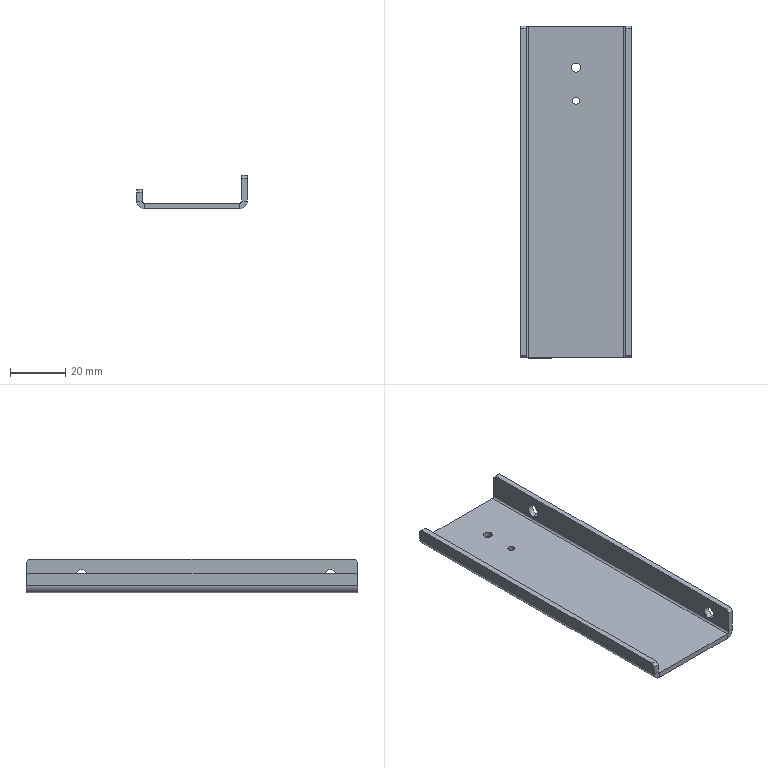Part | NX | features BREP 1 | 1 solid | 34 faces | box 40 x 120 x 12 mm | volume 12748 mm3 | plane 22 | cylinder 12 | commonest cylinder face diameters 4.5 x4 1.473 x2 2.5 x2 3.3 x2 5.473 x2
STEP:
#1=CARTESIAN_POINT('',(16.75,93.,-2.));
#2=VERTEX_POINT('',#1);
#3=CARTESIAN_POINT('',(19.25,93.,-2.));
#4=VERTEX_POINT('',#3);
#5=CARTESIAN_POINT('',(18.,93.,-2.));
#6=DIRECTION('',(0.,0.,1.));
#7=DIRECTION('',(1.,0.,0.));
#8=AXIS2_PLACEMENT_3D('',#5,#6,#7);
#9=CIRCLE('',#8,1.25);
#10=EDGE_CURVE('',#2,#4,#9,.T.);
#11=ORIENTED_EDGE('',*,*,#10,.F.);
#12=CARTESIAN_POINT('',(16.75,93.,0.));
#13=VERTEX_POINT('',#12);
#14=CARTESIAN_POINT('',(16.75,93.,0.));
#15=DIRECTION('',(0.,0.,1.));
#16=VECTOR('',#15,1000.);
#17=LINE('',#14,#16);
#18=EDGE_CURVE('',#13,#2,#17,.F.);
#19=ORIENTED_EDGE('',*,*,#18,.F.);
#20=CARTESIAN_POINT('',(19.25,93.,0.));
#21=VERTEX_POINT('',#20);
#22=CARTESIAN_POINT('',(18.,93.,0.));
#23=DIRECTION('',(0.,0.,1.));
#24=DIRECTION('',(1.,0.,0.));
#25=AXIS2_PLACEMENT_3D('',#22,#23,#24);
#26=CIRCLE('',#25,1.25);
#27=EDGE_CURVE('',#13,#21,#26,.T.);
#28=ORIENTED_EDGE('',*,*,#27,.T.);
#29=CARTESIAN_POINT('',(19.25,93.,0.));
#30=DIRECTION('',(0.,0.,1.));
#31=VECTOR('',#30,1000.);
#32=LINE('',#29,#31);
#33=EDGE_CURVE('',#21,#4,#32,.F.);
#34=ORIENTED_EDGE('',*,*,#33,.T.);
#35=EDGE_LOOP('',(#11,#19,#28,#34));
#36=FACE_BOUND('',#35,.T.);
#37=CARTESIAN_POINT('',(18.,93.,0.));
#38=DIRECTION('',(0.,0.,1.));
#39=DIRECTION('',(1.,0.,0.));
#40=AXIS2_PLACEMENT_3D('',#37,#38,#39);
#41=CYLINDRICAL_SURFACE('',#40,1.25);
#42=ADVANCED_FACE('',(#36),#41,.F.);
#43=CARTESIAN_POINT('',(16.35,105.,-2.));
#44=VERTEX_POINT('',#43);
#45=CARTESIAN_POINT('',(19.65,105.,-2.));
#46=VERTEX_POINT('',#45);
#47=CARTESIAN_POINT('',(18.,105.,-2.));
#48=DIRECTION('',(0.,0.,1.));
#49=DIRECTION('',(1.,0.,0.));
#50=AXIS2_PLACEMENT_3D('',#47,#48,#49);
#51=CIRCLE('',#50,1.65);
#52=EDGE_CURVE('',#44,#46,#51,.T.);
#53=ORIENTED_EDGE('',*,*,#52,.F.);
#54=CARTESIAN_POINT('',(16.35,105.,0.));
#55=VERTEX_POINT('',#54);
#56=CARTESIAN_POINT('',(16.35,105.,0.));
#57=DIRECTION('',(0.,0.,1.));
#58=VECTOR('',#57,1000.);
#59=LINE('',#56,#58);
#60=EDGE_CURVE('',#55,#44,#59,.F.);
#61=ORIENTED_EDGE('',*,*,#60,.F.);
#62=CARTESIAN_POINT('',(19.65,105.,0.));
#63=VERTEX_POINT('',#62);
#64=CARTESIAN_POINT('',(18.,105.,0.));
#65=DIRECTION('',(0.,0.,1.));
#66=DIRECTION('',(1.,0.,0.));
#67=AXIS2_PLACEMENT_3D('',#64,#65,#66);
#68=CIRCLE('',#67,1.65);
#69=EDGE_CURVE('',#55,#63,#68,.T.);
#70=ORIENTED_EDGE('',*,*,#69,.T.);
#71=CARTESIAN_POINT('',(19.65,105.,0.));
#72=DIRECTION('',(0.,0.,1.));
#73=VECTOR('',#72,1000.);
#74=LINE('',#71,#73);
#75=EDGE_CURVE('',#63,#46,#74,.F.);
#76=ORIENTED_EDGE('',*,*,#75,.T.);
#77=EDGE_LOOP('',(#53,#61,#70,#76));
#78=FACE_BOUND('',#77,.T.);
#79=CARTESIAN_POINT('',(18.,105.,0.));
#80=DIRECTION('',(0.,0.,1.));
#81=DIRECTION('',(1.,0.,0.));
#82=AXIS2_PLACEMENT_3D('',#79,#80,#81);
#83=CYLINDRICAL_SURFACE('',#82,1.65);
#84=ADVANCED_FACE('',(#78),#83,.F.);
#85=CARTESIAN_POINT('',(36.,100.,1.75));
#86=VERTEX_POINT('',#85);
#87=CARTESIAN_POINT('',(36.,100.,6.25));
#88=VERTEX_POINT('',#87);
#89=CARTESIAN_POINT('',(36.,100.,4.));
#90=DIRECTION('',(-1.,0.,0.));
#91=DIRECTION('',(0.,0.,1.));
#92=AXIS2_PLACEMENT_3D('',#89,#90,#91);
#93=CIRCLE('',#92,2.25);
#94=EDGE_CURVE('',#86,#88,#93,.T.);
#95=ORIENTED_EDGE('',*,*,#94,.T.);
#96=CARTESIAN_POINT('',(38.,100.,6.25));
#97=VERTEX_POINT('',#96);
#98=CARTESIAN_POINT('',(38.,100.,6.25));
#99=DIRECTION('',(1.,0.,0.));
#100=VECTOR('',#99,1000.);
#101=LINE('',#98,#100);
#102=EDGE_CURVE('',#88,#97,#101,.T.);
#103=ORIENTED_EDGE('',*,*,#102,.T.);
#104=CARTESIAN_POINT('',(38.,100.,1.75));
#105=VERTEX_POINT('',#104);
#106=CARTESIAN_POINT('',(38.,100.,4.));
#107=DIRECTION('',(1.,0.,0.));
#108=DIRECTION('',(0.,0.,-1.));
#109=AXIS2_PLACEMENT_3D('',#106,#107,#108);
#110=CIRCLE('',#109,2.25);
#111=EDGE_CURVE('',#97,#105,#110,.T.);
#112=ORIENTED_EDGE('',*,*,#111,.T.);
#113=CARTESIAN_POINT('',(38.,100.,1.75));
#114=DIRECTION('',(1.,0.,0.));
#115=VECTOR('',#114,1000.);
#116=LINE('',#113,#115);
#117=EDGE_CURVE('',#86,#105,#116,.T.);
#118=ORIENTED_EDGE('',*,*,#117,.F.);
#119=EDGE_LOOP('',(#95,#103,#112,#118));
#120=FACE_BOUND('',#119,.T.);
#121=CARTESIAN_POINT('',(38.,100.,4.));
#122=DIRECTION('',(1.,0.,0.));
#123=DIRECTION('',(0.,0.,-1.));
#124=AXIS2_PLACEMENT_3D('',#121,#122,#123);
#125=CYLINDRICAL_SURFACE('',#124,2.25);
#126=ADVANCED_FACE('',(#120),#125,.F.);
#127=CARTESIAN_POINT('',(36.,10.,1.75));
#128=VERTEX_POINT('',#127);
#129=CARTESIAN_POINT('',(36.,10.,6.25));
#130=VERTEX_POINT('',#129);
#131=CARTESIAN_POINT('',(36.,10.,4.));
#132=DIRECTION('',(-1.,0.,0.));
#133=DIRECTION('',(0.,0.,1.));
#134=AXIS2_PLACEMENT_3D('',#131,#132,#133);
#135=CIRCLE('',#134,2.25);
#136=EDGE_CURVE('',#128,#130,#135,.T.);
#137=ORIENTED_EDGE('',*,*,#136,.T.);
#138=CARTESIAN_POINT('',(38.,10.,6.25));
#139=VERTEX_POINT('',#138);
#140=CARTESIAN_POINT('',(38.,10.,6.25));
#141=DIRECTION('',(1.,0.,0.));
#142=VECTOR('',#141,1000.);
#143=LINE('',#140,#142);
#144=EDGE_CURVE('',#130,#139,#143,.T.);
#145=ORIENTED_EDGE('',*,*,#144,.T.);
#146=CARTESIAN_POINT('',(38.,10.,1.75));
#147=VERTEX_POINT('',#146);
#148=CARTESIAN_POINT('',(38.,10.,4.));
#149=DIRECTION('',(1.,0.,0.));
#150=DIRECTION('',(0.,0.,-1.));
#151=AXIS2_PLACEMENT_3D('',#148,#149,#150);
#152=CIRCLE('',#151,2.25);
#153=EDGE_CURVE('',#139,#147,#152,.T.);
#154=ORIENTED_EDGE('',*,*,#153,.T.);
#155=CARTESIAN_POINT('',(38.,10.,1.75));
#156=DIRECTION('',(1.,0.,0.));
#157=VECTOR('',#156,1000.);
#158=LINE('',#155,#157);
#159=EDGE_CURVE('',#128,#147,#158,.T.);
#160=ORIENTED_EDGE('',*,*,#159,.F.);
#161=EDGE_LOOP('',(#137,#145,#154,#160));
#162=FACE_BOUND('',#161,.T.);
#163=CARTESIAN_POINT('',(38.,10.,4.));
#164=DIRECTION('',(1.,0.,0.));
#165=DIRECTION('',(0.,0.,-1.));
#166=AXIS2_PLACEMENT_3D('',#163,#164,#165);
#167=CYLINDRICAL_SURFACE('',#166,2.25);
#168=ADVANCED_FACE('',(#162),#167,.F.);
#169=CARTESIAN_POINT('',(38.,119.,10.));
#170=VERTEX_POINT('',#169);
#171=CARTESIAN_POINT('',(38.,1.,10.));
#172=VERTEX_POINT('',#171);
#173=CARTESIAN_POINT('',(38.,0.,10.));
#174=DIRECTION('',(0.,-1.,0.));
#175=VECTOR('',#174,1000.);
#176=LINE('',#173,#175);
#177=EDGE_CURVE('',#170,#172,#176,.T.);
#178=ORIENTED_EDGE('',*,*,#177,.T.);
#179=CARTESIAN_POINT('',(38.,0.,9.));
#180=VERTEX_POINT('',#179);
#181=CARTESIAN_POINT('',(38.,0.,9.));
#182=DIRECTION('',(0.,-0.7071,-0.7071));
#183=VECTOR('',#182,1000.);
#184=LINE('',#181,#183);
#185=EDGE_CURVE('',#172,#180,#184,.T.);
#186=ORIENTED_EDGE('',*,*,#185,.T.);
#187=CARTESIAN_POINT('',(38.,0.,0.7366));
#188=VERTEX_POINT('',#187);
#189=CARTESIAN_POINT('',(38.,0.,0.));
#190=DIRECTION('',(0.,0.,-1.));
#191=VECTOR('',#190,1000.);
#192=LINE('',#189,#191);
#193=EDGE_CURVE('',#180,#188,#192,.T.);
#194=ORIENTED_EDGE('',*,*,#193,.T.);
#195=CARTESIAN_POINT('',(38.,120.,0.7366));
#196=VERTEX_POINT('',#195);
#197=CARTESIAN_POINT('',(38.,0.,0.7366));
#198=DIRECTION('',(0.,-1.,0.));
#199=VECTOR('',#198,1000.);
#200=LINE('',#197,#199);
#201=EDGE_CURVE('',#196,#188,#200,.T.);
#202=ORIENTED_EDGE('',*,*,#201,.F.);
#203=CARTESIAN_POINT('',(38.,120.,9.));
#204=VERTEX_POINT('',#203);
#205=CARTESIAN_POINT('',(38.,120.,10.));
#206=DIRECTION('',(0.,0.,1.));
#207=VECTOR('',#206,1000.);
#208=LINE('',#205,#207);
#209=EDGE_CURVE('',#196,#204,#208,.T.);
#210=ORIENTED_EDGE('',*,*,#209,.T.);
#211=CARTESIAN_POINT('',(38.,119.,10.));
#212=DIRECTION('',(0.,-0.7071,0.7071));
#213=VECTOR('',#212,1000.);
#214=LINE('',#211,#213);
#215=EDGE_CURVE('',#204,#170,#214,.T.);
#216=ORIENTED_EDGE('',*,*,#215,.T.);
#217=EDGE_LOOP('',(#178,#186,#194,#202,#210,#216));
#218=FACE_BOUND('',#217,.T.);
#219=CARTESIAN_POINT('',(38.,10.,4.));
#220=DIRECTION('',(1.,0.,0.));
#221=DIRECTION('',(0.,0.,-1.));
#222=AXIS2_PLACEMENT_3D('',#219,#220,#221);
#223=CIRCLE('',#222,2.25);
#224=EDGE_CURVE('',#147,#139,#223,.T.);
#225=ORIENTED_EDGE('',*,*,#224,.F.);
#226=ORIENTED_EDGE('',*,*,#153,.F.);
#227=EDGE_LOOP('',(#225,#226));
#228=FACE_BOUND('',#227,.T.);
#229=CARTESIAN_POINT('',(38.,100.,4.));
#230=DIRECTION('',(1.,0.,0.));
#231=DIRECTION('',(0.,0.,-1.));
#232=AXIS2_PLACEMENT_3D('',#229,#230,#231);
#233=CIRCLE('',#232,2.25);
#234=EDGE_CURVE('',#105,#97,#233,.T.);
#235=ORIENTED_EDGE('',*,*,#234,.F.);
#236=ORIENTED_EDGE('',*,*,#111,.F.);
#237=EDGE_LOOP('',(#235,#236));
#238=FACE_BOUND('',#237,.T.);
#239=CARTESIAN_POINT('',(38.,0.,0.));
#240=DIRECTION('',(-1.,0.,0.));
#241=DIRECTION('',(0.,1.,0.));
#242=AXIS2_PLACEMENT_3D('',#239,#240,#241);
#243=PLANE('',#242);
#244=ADVANCED_FACE('',(#218,#228,#238),#243,.F.);
#245=CARTESIAN_POINT('',(35.263,120.,-2.));
#246=VERTEX_POINT('',#245);
#247=CARTESIAN_POINT('',(0.7366,120.,-2.));
#248=VERTEX_POINT('',#247);
#249=CARTESIAN_POINT('',(0.,120.,-2.));
#250=DIRECTION('',(-1.,0.,0.));
#251=VECTOR('',#250,1000.);
#252=LINE('',#249,#251);
#253=EDGE_CURVE('',#246,#248,#252,.T.);
#254=ORIENTED_EDGE('',*,*,#253,.F.);
#255=CARTESIAN_POINT('',(35.263,0.,-2.));
#256=VERTEX_POINT('',#255);
#257=CARTESIAN_POINT('',(35.263,120.,-2.));
#258=DIRECTION('',(0.,-1.,0.));
#259=VECTOR('',#258,1000.);
#260=LINE('',#257,#259);
#261=EDGE_CURVE('',#246,#256,#260,.T.);
#262=ORIENTED_EDGE('',*,*,#261,.T.);
#263=CARTESIAN_POINT('',(0.7366,0.,-2.));
#264=VERTEX_POINT('',#263);
#265=CARTESIAN_POINT('',(0.,0.,-2.));
#266=DIRECTION('',(1.,0.,0.));
#267=VECTOR('',#266,1000.);
#268=LINE('',#265,#267);
#269=EDGE_CURVE('',#264,#256,#268,.T.);
#270=ORIENTED_EDGE('',*,*,#269,.F.);
#271=CARTESIAN_POINT('',(0.7366,0.,-2.));
#272=DIRECTION('',(0.,1.,0.));
#273=VECTOR('',#272,1000.);
#274=LINE('',#271,#273);
#275=EDGE_CURVE('',#264,#248,#274,.T.);
#276=ORIENTED_EDGE('',*,*,#275,.T.);
#277=EDGE_LOOP('',(#254,#262,#270,#276));
#278=FACE_BOUND('',#277,.T.);
#279=CARTESIAN_POINT('',(18.,93.,-2.));
#280=DIRECTION('',(0.,0.,1.));
#281=DIRECTION('',(1.,0.,0.));
#282=AXIS2_PLACEMENT_3D('',#279,#280,#281);
#283=CIRCLE('',#282,1.25);
#284=EDGE_CURVE('',#4,#2,#283,.T.);
#285=ORIENTED_EDGE('',*,*,#284,.T.);
#286=ORIENTED_EDGE('',*,*,#10,.T.);
#287=EDGE_LOOP('',(#285,#286));
#288=FACE_BOUND('',#287,.T.);
#289=CARTESIAN_POINT('',(18.,105.,-2.));
#290=DIRECTION('',(0.,0.,1.));
#291=DIRECTION('',(1.,0.,0.));
#292=AXIS2_PLACEMENT_3D('',#289,#290,#291);
#293=CIRCLE('',#292,1.65);
#294=EDGE_CURVE('',#46,#44,#293,.T.);
#295=ORIENTED_EDGE('',*,*,#294,.T.);
#296=ORIENTED_EDGE('',*,*,#52,.T.);
#297=EDGE_LOOP('',(#295,#296));
#298=FACE_BOUND('',#297,.T.);
#299=CARTESIAN_POINT('',(0.,0.,-2.));
#300=DIRECTION('',(0.,0.,-1.));
#301=DIRECTION('',(0.,-1.,0.));
#302=AXIS2_PLACEMENT_3D('',#299,#300,#301);
#303=PLANE('',#302);
#304=ADVANCED_FACE('',(#278,#288,#298),#303,.T.);
#305=CARTESIAN_POINT('',(35.263,120.,0.));
#306=VERTEX_POINT('',#305);
#307=CARTESIAN_POINT('',(35.263,0.,0.));
#308=VERTEX_POINT('',#307);
#309=CARTESIAN_POINT('',(35.263,120.,0.));
#310=DIRECTION('',(0.,-1.,0.));
#311=VECTOR('',#310,1000.);
#312=LINE('',#309,#311);
#313=EDGE_CURVE('',#306,#308,#312,.T.);
#314=ORIENTED_EDGE('',*,*,#313,.F.);
#315=CARTESIAN_POINT('',(0.7366,120.,0.));
#316=VERTEX_POINT('',#315);
#317=CARTESIAN_POINT('',(0.,120.,0.));
#318=DIRECTION('',(-1.,0.,0.));
#319=VECTOR('',#318,1000.);
#320=LINE('',#317,#319);
#321=EDGE_CURVE('',#306,#316,#320,.T.);
#322=ORIENTED_EDGE('',*,*,#321,.T.);
#323=CARTESIAN_POINT('',(0.7366,0.,0.));
#324=VERTEX_POINT('',#323);
#325=CARTESIAN_POINT('',(0.7366,0.,0.));
#326=DIRECTION('',(0.,1.,0.));
#327=VECTOR('',#326,1000.);
#328=LINE('',#325,#327);
#329=EDGE_CURVE('',#324,#316,#328,.T.);
#330=ORIENTED_EDGE('',*,*,#329,.F.);
#331=CARTESIAN_POINT('',(0.,0.,0.));
#332=DIRECTION('',(1.,0.,0.));
#333=VECTOR('',#332,1000.);
#334=LINE('',#331,#333);
#335=EDGE_CURVE('',#324,#308,#334,.T.);
#336=ORIENTED_EDGE('',*,*,#335,.T.);
#337=EDGE_LOOP('',(#314,#322,#330,#336));
#338=FACE_BOUND('',#337,.T.);
#339=CARTESIAN_POINT('',(18.,93.,0.));
#340=DIRECTION('',(0.,0.,1.));
#341=DIRECTION('',(1.,0.,0.));
#342=AXIS2_PLACEMENT_3D('',#339,#340,#341);
#343=CIRCLE('',#342,1.25);
#344=EDGE_CURVE('',#21,#13,#343,.T.);
#345=ORIENTED_EDGE('',*,*,#344,.F.);
#346=ORIENTED_EDGE('',*,*,#27,.F.);
#347=EDGE_LOOP('',(#345,#346));
#348=FACE_BOUND('',#347,.T.);
#349=CARTESIAN_POINT('',(18.,105.,0.));
#350=DIRECTION('',(0.,0.,1.));
#351=DIRECTION('',(1.,0.,0.));
#352=AXIS2_PLACEMENT_3D('',#349,#350,#351);
#353=CIRCLE('',#352,1.65);
#354=EDGE_CURVE('',#63,#55,#353,.T.);
#355=ORIENTED_EDGE('',*,*,#354,.F.);
#356=ORIENTED_EDGE('',*,*,#69,.F.);
#357=EDGE_LOOP('',(#355,#356));
#358=FACE_BOUND('',#357,.T.);
#359=CARTESIAN_POINT('',(0.,0.,0.));
#360=DIRECTION('',(0.,0.,-1.));
#361=DIRECTION('',(0.,-1.,0.));
#362=AXIS2_PLACEMENT_3D('',#359,#360,#361);
#363=PLANE('',#362);
#364=ADVANCED_FACE('',(#338,#348,#358),#363,.F.);
#365=ORIENTED_EDGE('',*,*,#321,.F.);
#366=CARTESIAN_POINT('',(35.263,120.,0.));
#367=DIRECTION('',(0.,0.,-1.));
#368=VECTOR('',#367,1000.);
#369=LINE('',#366,#368);
#370=EDGE_CURVE('',#306,#246,#369,.T.);
#371=ORIENTED_EDGE('',*,*,#370,.T.);
#372=ORIENTED_EDGE('',*,*,#253,.T.);
#373=CARTESIAN_POINT('',(0.7366,120.,0.));
#374=DIRECTION('',(0.,0.,-1.));
#375=VECTOR('',#374,1000.);
#376=LINE('',#373,#375);
#377=EDGE_CURVE('',#316,#248,#376,.T.);
#378=ORIENTED_EDGE('',*,*,#377,.F.);
#379=EDGE_LOOP('',(#365,#371,#372,#378));
#380=FACE_BOUND('',#379,.T.);
#381=CARTESIAN_POINT('',(0.,120.,-2.));
#382=DIRECTION('',(0.,1.,0.));
#383=DIRECTION('',(1.,0.,0.));
#384=AXIS2_PLACEMENT_3D('',#381,#382,#383);
#385=PLANE('',#384);
#386=ADVANCED_FACE('',(#380),#385,.T.);
#387=CARTESIAN_POINT('',(35.263,0.,0.));
#388=DIRECTION('',(0.,0.,-1.));
#389=VECTOR('',#388,1000.);
#390=LINE('',#387,#389);
#391=EDGE_CURVE('',#308,#256,#390,.T.);
#392=ORIENTED_EDGE('',*,*,#391,.F.);
#393=ORIENTED_EDGE('',*,*,#335,.F.);
#394=CARTESIAN_POINT('',(0.7366,0.,0.));
#395=DIRECTION('',(0.,0.,-1.));
#396=VECTOR('',#395,1000.);
#397=LINE('',#394,#396);
#398=EDGE_CURVE('',#324,#264,#397,.T.);
#399=ORIENTED_EDGE('',*,*,#398,.T.);
#400=ORIENTED_EDGE('',*,*,#269,.T.);
#401=EDGE_LOOP('',(#392,#393,#399,#400));
#402=FACE_BOUND('',#401,.T.);
#403=CARTESIAN_POINT('',(0.,0.,-2.));
#404=DIRECTION('',(0.,-1.,0.));
#405=DIRECTION('',(0.,0.,-1.));
#406=AXIS2_PLACEMENT_3D('',#403,#404,#405);
#407=PLANE('',#406);
#408=ADVANCED_FACE('',(#402),#407,.T.);
#409=CARTESIAN_POINT('',(0.,120.,0.7366));
#410=VERTEX_POINT('',#409);
#411=CARTESIAN_POINT('',(-2.,120.,0.7366));
#412=VERTEX_POINT('',#411);
#413=CARTESIAN_POINT('',(0.,120.,0.7366));
#414=DIRECTION('',(-1.,0.,0.));
#415=VECTOR('',#414,1000.);
#416=LINE('',#413,#415);
#417=EDGE_CURVE('',#410,#412,#416,.T.);
#418=ORIENTED_EDGE('',*,*,#417,.F.);
#419=CARTESIAN_POINT('',(0.7366,120.,0.7366));
#420=DIRECTION('',(0.,1.,0.));
#421=DIRECTION('',(1.,0.,0.));
#422=AXIS2_PLACEMENT_3D('',#419,#420,#421);
#423=CIRCLE('',#422,0.7366);
#424=EDGE_CURVE('',#316,#410,#423,.T.);
#425=ORIENTED_EDGE('',*,*,#424,.F.);
#426=ORIENTED_EDGE('',*,*,#377,.T.);
#427=CARTESIAN_POINT('',(0.7366,120.,0.7366));
#428=DIRECTION('',(0.,1.,0.));
#429=DIRECTION('',(1.,0.,0.));
#430=AXIS2_PLACEMENT_3D('',#427,#428,#429);
#431=CIRCLE('',#430,2.737);
#432=EDGE_CURVE('',#248,#412,#431,.T.);
#433=ORIENTED_EDGE('',*,*,#432,.T.);
#434=EDGE_LOOP('',(#418,#425,#426,#433));
#435=FACE_BOUND('',#434,.T.);
#436=CARTESIAN_POINT('',(0.7366,120.,0.7366));
#437=DIRECTION('',(0.,1.,0.));
#438=DIRECTION('',(1.,0.,0.));
#439=AXIS2_PLACEMENT_3D('',#436,#437,#438);
#440=PLANE('',#439);
#441=ADVANCED_FACE('',(#435),#440,.T.);
#442=CARTESIAN_POINT('',(0.,0.,0.7366));
#443=VERTEX_POINT('',#442);
#444=CARTESIAN_POINT('',(0.7366,0.,0.7366));
#445=DIRECTION('',(0.,-1.,0.));
#446=DIRECTION('',(1.,0.,0.));
#447=AXIS2_PLACEMENT_3D('',#444,#445,#446);
#448=CIRCLE('',#447,0.7366);
#449=EDGE_CURVE('',#443,#324,#448,.T.);
#450=ORIENTED_EDGE('',*,*,#449,.F.);
#451=CARTESIAN_POINT('',(-2.,0.,0.7366));
#452=VERTEX_POINT('',#451);
#453=CARTESIAN_POINT('',(0.,0.,0.7366));
#454=DIRECTION('',(-1.,0.,0.));
#455=VECTOR('',#454,1000.);
#456=LINE('',#453,#455);
#457=EDGE_CURVE('',#443,#452,#456,.T.);
#458=ORIENTED_EDGE('',*,*,#457,.T.);
#459=CARTESIAN_POINT('',(0.7366,0.,0.7366));
#460=DIRECTION('',(0.,-1.,0.));
#461=DIRECTION('',(1.,0.,0.));
#462=AXIS2_PLACEMENT_3D('',#459,#460,#461);
#463=CIRCLE('',#462,2.737);
#464=EDGE_CURVE('',#452,#264,#463,.T.);
#465=ORIENTED_EDGE('',*,*,#464,.T.);
#466=ORIENTED_EDGE('',*,*,#398,.F.);
#467=EDGE_LOOP('',(#450,#458,#465,#466));
#468=FACE_BOUND('',#467,.T.);
#469=CARTESIAN_POINT('',(0.7366,0.,0.7366));
#470=DIRECTION('',(0.,1.,0.));
#471=DIRECTION('',(1.,0.,0.));
#472=AXIS2_PLACEMENT_3D('',#469,#470,#471);
#473=PLANE('',#472);
#474=ADVANCED_FACE('',(#468),#473,.F.);
#475=ORIENTED_EDGE('',*,*,#275,.F.);
#476=ORIENTED_EDGE('',*,*,#464,.F.);
#477=CARTESIAN_POINT('',(-2.,0.,0.7366));
#478=DIRECTION('',(0.,1.,0.));
#479=VECTOR('',#478,1000.);
#480=LINE('',#477,#479);
#481=EDGE_CURVE('',#452,#412,#480,.T.);
#482=ORIENTED_EDGE('',*,*,#481,.T.);
#483=ORIENTED_EDGE('',*,*,#432,.F.);
#484=EDGE_LOOP('',(#475,#476,#482,#483));
#485=FACE_BOUND('',#484,.T.);
#486=CARTESIAN_POINT('',(0.7366,0.,0.7366));
#487=DIRECTION('',(0.,-1.,0.));
#488=DIRECTION('',(-1.,0.,0.));
#489=AXIS2_PLACEMENT_3D('',#486,#487,#488);
#490=CYLINDRICAL_SURFACE('',#489,2.737);
#491=ADVANCED_FACE('',(#485),#490,.T.);
#492=ORIENTED_EDGE('',*,*,#329,.T.);
#493=ORIENTED_EDGE('',*,*,#424,.T.);
#494=CARTESIAN_POINT('',(0.,120.,0.7366));
#495=DIRECTION('',(0.,-1.,0.));
#496=VECTOR('',#495,1000.);
#497=LINE('',#494,#496);
#498=EDGE_CURVE('',#410,#443,#497,.T.);
#499=ORIENTED_EDGE('',*,*,#498,.T.);
#500=ORIENTED_EDGE('',*,*,#449,.T.);
#501=EDGE_LOOP('',(#492,#493,#499,#500));
#502=FACE_BOUND('',#501,.T.);
#503=CARTESIAN_POINT('',(0.7366,0.,0.7366));
#504=DIRECTION('',(0.,-1.,0.));
#505=DIRECTION('',(-1.,0.,0.));
#506=AXIS2_PLACEMENT_3D('',#503,#504,#505);
#507=CYLINDRICAL_SURFACE('',#506,0.7366);
#508=ADVANCED_FACE('',(#502),#507,.F.);
#509=CARTESIAN_POINT('',(0.,0.,4.));
#510=VERTEX_POINT('',#509);
#511=CARTESIAN_POINT('',(0.,0.,5.));
#512=DIRECTION('',(0.,0.,1.));
#513=VECTOR('',#512,1000.);
#514=LINE('',#511,#513);
#515=EDGE_CURVE('',#443,#510,#514,.T.);
#516=ORIENTED_EDGE('',*,*,#515,.T.);
#517=CARTESIAN_POINT('',(-2.,0.,4.));
#518=VERTEX_POINT('',#517);
#519=CARTESIAN_POINT('',(-2.,0.,4.));
#520=DIRECTION('',(-1.,0.,0.));
#521=VECTOR('',#520,1000.);
#522=LINE('',#519,#521);
#523=EDGE_CURVE('',#510,#518,#522,.T.);
#524=ORIENTED_EDGE('',*,*,#523,.T.);
#525=CARTESIAN_POINT('',(-2.,0.,5.));
#526=DIRECTION('',(0.,0.,1.));
#527=VECTOR('',#526,1000.);
#528=LINE('',#525,#527);
#529=EDGE_CURVE('',#452,#518,#528,.T.);
#530=ORIENTED_EDGE('',*,*,#529,.F.);
#531=ORIENTED_EDGE('',*,*,#457,.F.);
#532=EDGE_LOOP('',(#516,#524,#530,#531));
#533=FACE_BOUND('',#532,.T.);
#534=CARTESIAN_POINT('',(-2.,0.,5.));
#535=DIRECTION('',(0.,1.,0.));
#536=DIRECTION('',(1.,0.,0.));
#537=AXIS2_PLACEMENT_3D('',#534,#535,#536);
#538=PLANE('',#537);
#539=ADVANCED_FACE('',(#533),#538,.F.);
#540=CARTESIAN_POINT('',(-2.,120.,4.));
#541=VERTEX_POINT('',#540);
#542=CARTESIAN_POINT('',(-2.,120.,0.));
#543=DIRECTION('',(0.,0.,-1.));
#544=VECTOR('',#543,1000.);
#545=LINE('',#542,#544);
#546=EDGE_CURVE('',#541,#412,#545,.T.);
#547=ORIENTED_EDGE('',*,*,#546,.F.);
#548=CARTESIAN_POINT('',(0.,120.,4.));
#549=VERTEX_POINT('',#548);
#550=CARTESIAN_POINT('',(-2.,120.,4.));
#551=DIRECTION('',(1.,0.,0.));
#552=VECTOR('',#551,1000.);
#553=LINE('',#550,#552);
#554=EDGE_CURVE('',#541,#549,#553,.T.);
#555=ORIENTED_EDGE('',*,*,#554,.T.);
#556=CARTESIAN_POINT('',(0.,120.,0.));
#557=DIRECTION('',(0.,0.,-1.));
#558=VECTOR('',#557,1000.);
#559=LINE('',#556,#558);
#560=EDGE_CURVE('',#549,#410,#559,.T.);
#561=ORIENTED_EDGE('',*,*,#560,.T.);
#562=ORIENTED_EDGE('',*,*,#417,.T.);
#563=EDGE_LOOP('',(#547,#555,#561,#562));
#564=FACE_BOUND('',#563,.T.);
#565=CARTESIAN_POINT('',(-2.,120.,0.));
#566=DIRECTION('',(0.,-1.,0.));
#567=DIRECTION('',(0.,0.,-1.));
#568=AXIS2_PLACEMENT_3D('',#565,#566,#567);
#569=PLANE('',#568);
#570=ADVANCED_FACE('',(#564),#569,.F.);
#571=CARTESIAN_POINT('',(-2.,1.,5.));
#572=VERTEX_POINT('',#571);
#573=CARTESIAN_POINT('',(-2.,119.,5.));
#574=VERTEX_POINT('',#573);
#575=CARTESIAN_POINT('',(-2.,120.,5.));
#576=DIRECTION('',(0.,1.,0.));
#577=VECTOR('',#576,1000.);
#578=LINE('',#575,#577);
#579=EDGE_CURVE('',#572,#574,#578,.T.);
#580=ORIENTED_EDGE('',*,*,#579,.T.);
#581=CARTESIAN_POINT('',(-2.,120.,4.));
#582=DIRECTION('',(0.,0.7071,-0.7071));
#583=VECTOR('',#582,1000.);
#584=LINE('',#581,#583);
#585=EDGE_CURVE('',#574,#541,#584,.T.);
#586=ORIENTED_EDGE('',*,*,#585,.T.);
#587=ORIENTED_EDGE('',*,*,#546,.T.);
#588=ORIENTED_EDGE('',*,*,#481,.F.);
#589=ORIENTED_EDGE('',*,*,#529,.T.);
#590=CARTESIAN_POINT('',(-2.,1.,5.));
#591=DIRECTION('',(0.,0.7071,0.7071));
#592=VECTOR('',#591,1000.);
#593=LINE('',#590,#592);
#594=EDGE_CURVE('',#518,#572,#593,.T.);
#595=ORIENTED_EDGE('',*,*,#594,.T.);
#596=EDGE_LOOP('',(#580,#586,#587,#588,#589,#595));
#597=FACE_BOUND('',#596,.T.);
#598=CARTESIAN_POINT('',(-2.,0.,0.));
#599=DIRECTION('',(1.,0.,0.));
#600=DIRECTION('',(0.,0.,1.));
#601=AXIS2_PLACEMENT_3D('',#598,#599,#600);
#602=PLANE('',#601);
#603=ADVANCED_FACE('',(#597),#602,.F.);
#604=ORIENTED_EDGE('',*,*,#560,.F.);
#605=CARTESIAN_POINT('',(0.,119.,5.));
#606=VERTEX_POINT('',#605);
#607=CARTESIAN_POINT('',(0.,62.,62.));
#608=DIRECTION('',(0.,-0.7071,0.7071));
#609=VECTOR('',#608,1000.);
#610=LINE('',#607,#609);
#611=EDGE_CURVE('',#549,#606,#610,.T.);
#612=ORIENTED_EDGE('',*,*,#611,.T.);
#613=CARTESIAN_POINT('',(0.,1.,5.));
#614=VERTEX_POINT('',#613);
#615=CARTESIAN_POINT('',(0.,120.,5.));
#616=DIRECTION('',(0.,1.,0.));
#617=VECTOR('',#616,1000.);
#618=LINE('',#615,#617);
#619=EDGE_CURVE('',#614,#606,#618,.T.);
#620=ORIENTED_EDGE('',*,*,#619,.F.);
#621=CARTESIAN_POINT('',(0.,-2.,2.));
#622=DIRECTION('',(0.,-0.7071,-0.7071));
#623=VECTOR('',#622,1000.);
#624=LINE('',#621,#623);
#625=EDGE_CURVE('',#614,#510,#624,.T.);
#626=ORIENTED_EDGE('',*,*,#625,.T.);
#627=ORIENTED_EDGE('',*,*,#515,.F.);
#628=ORIENTED_EDGE('',*,*,#498,.F.);
#629=EDGE_LOOP('',(#604,#612,#620,#626,#627,#628));
#630=FACE_BOUND('',#629,.T.);
#631=CARTESIAN_POINT('',(0.,0.,0.));
#632=DIRECTION('',(1.,0.,0.));
#633=DIRECTION('',(0.,0.,1.));
#634=AXIS2_PLACEMENT_3D('',#631,#632,#633);
#635=PLANE('',#634);
#636=ADVANCED_FACE('',(#630),#635,.T.);
#637=ORIENTED_EDGE('',*,*,#619,.T.);
#638=CARTESIAN_POINT('',(-2.,119.,5.));
#639=DIRECTION('',(-1.,0.,0.));
#640=VECTOR('',#639,1000.);
#641=LINE('',#638,#640);
#642=EDGE_CURVE('',#606,#574,#641,.T.);
#643=ORIENTED_EDGE('',*,*,#642,.T.);
#644=ORIENTED_EDGE('',*,*,#579,.F.);
#645=CARTESIAN_POINT('',(-2.,1.,5.));
#646=DIRECTION('',(1.,0.,0.));
#647=VECTOR('',#646,1000.);
#648=LINE('',#645,#647);
#649=EDGE_CURVE('',#572,#614,#648,.T.);
#650=ORIENTED_EDGE('',*,*,#649,.T.);
#651=EDGE_LOOP('',(#637,#643,#644,#650));
#652=FACE_BOUND('',#651,.T.);
#653=CARTESIAN_POINT('',(-2.,120.,5.));
#654=DIRECTION('',(0.,0.,-1.));
#655=DIRECTION('',(0.,-1.,0.));
#656=AXIS2_PLACEMENT_3D('',#653,#654,#655);
#657=PLANE('',#656);
#658=ADVANCED_FACE('',(#652),#657,.F.);
#659=CARTESIAN_POINT('',(36.,0.,0.7366));
#660=VERTEX_POINT('',#659);
#661=CARTESIAN_POINT('',(36.,0.,0.7366));
#662=DIRECTION('',(1.,0.,0.));
#663=VECTOR('',#662,1000.);
#664=LINE('',#661,#663);
#665=EDGE_CURVE('',#660,#188,#664,.T.);
#666=ORIENTED_EDGE('',*,*,#665,.F.);
#667=CARTESIAN_POINT('',(35.263,0.,0.7366));
#668=DIRECTION('',(0.,-1.,0.));
#669=DIRECTION('',(0.,0.,1.));
#670=AXIS2_PLACEMENT_3D('',#667,#668,#669);
#671=CIRCLE('',#670,0.7366);
#672=EDGE_CURVE('',#308,#660,#671,.T.);
#673=ORIENTED_EDGE('',*,*,#672,.F.);
#674=ORIENTED_EDGE('',*,*,#391,.T.);
#675=CARTESIAN_POINT('',(35.263,0.,0.7366));
#676=DIRECTION('',(0.,-1.,0.));
#677=DIRECTION('',(0.,0.,1.));
#678=AXIS2_PLACEMENT_3D('',#675,#676,#677);
#679=CIRCLE('',#678,2.737);
#680=EDGE_CURVE('',#256,#188,#679,.T.);
#681=ORIENTED_EDGE('',*,*,#680,.T.);
#682=EDGE_LOOP('',(#666,#673,#674,#681));
#683=FACE_BOUND('',#682,.T.);
#684=CARTESIAN_POINT('',(35.263,0.,0.7366));
#685=DIRECTION('',(0.,-1.,0.));
#686=DIRECTION('',(0.,0.,-1.));
#687=AXIS2_PLACEMENT_3D('',#684,#685,#686);
#688=PLANE('',#687);
#689=ADVANCED_FACE('',(#683),#688,.T.);
#690=CARTESIAN_POINT('',(36.,120.,0.7366));
#691=VERTEX_POINT('',#690);
#692=CARTESIAN_POINT('',(35.263,120.,0.7366));
#693=DIRECTION('',(0.,1.,0.));
#694=DIRECTION('',(0.,0.,1.));
#695=AXIS2_PLACEMENT_3D('',#692,#693,#694);
#696=CIRCLE('',#695,0.7366);
#697=EDGE_CURVE('',#691,#306,#696,.T.);
#698=ORIENTED_EDGE('',*,*,#697,.F.);
#699=CARTESIAN_POINT('',(36.,120.,0.7366));
#700=DIRECTION('',(1.,0.,0.));
#701=VECTOR('',#700,1000.);
#702=LINE('',#699,#701);
#703=EDGE_CURVE('',#691,#196,#702,.T.);
#704=ORIENTED_EDGE('',*,*,#703,.T.);
#705=CARTESIAN_POINT('',(35.263,120.,0.7366));
#706=DIRECTION('',(0.,1.,0.));
#707=DIRECTION('',(0.,0.,1.));
#708=AXIS2_PLACEMENT_3D('',#705,#706,#707);
#709=CIRCLE('',#708,2.737);
#710=EDGE_CURVE('',#196,#246,#709,.T.);
#711=ORIENTED_EDGE('',*,*,#710,.T.);
#712=ORIENTED_EDGE('',*,*,#370,.F.);
#713=EDGE_LOOP('',(#698,#704,#711,#712));
#714=FACE_BOUND('',#713,.T.);
#715=CARTESIAN_POINT('',(35.263,120.,0.7366));
#716=DIRECTION('',(0.,-1.,0.));
#717=DIRECTION('',(0.,0.,-1.));
#718=AXIS2_PLACEMENT_3D('',#715,#716,#717);
#719=PLANE('',#718);
#720=ADVANCED_FACE('',(#714),#719,.F.);
#721=ORIENTED_EDGE('',*,*,#261,.F.);
#722=ORIENTED_EDGE('',*,*,#710,.F.);
#723=ORIENTED_EDGE('',*,*,#201,.T.);
#724=ORIENTED_EDGE('',*,*,#680,.F.);
#725=EDGE_LOOP('',(#721,#722,#723,#724));
#726=FACE_BOUND('',#725,.T.);
#727=CARTESIAN_POINT('',(35.263,120.,0.7366));
#728=DIRECTION('',(0.,1.,0.));
#729=DIRECTION('',(1.,0.,0.));
#730=AXIS2_PLACEMENT_3D('',#727,#728,#729);
#731=CYLINDRICAL_SURFACE('',#730,2.737);
#732=ADVANCED_FACE('',(#726),#731,.T.);
#733=ORIENTED_EDGE('',*,*,#313,.T.);
#734=ORIENTED_EDGE('',*,*,#672,.T.);
#735=CARTESIAN_POINT('',(36.,0.,0.7366));
#736=DIRECTION('',(0.,1.,0.));
#737=VECTOR('',#736,1000.);
#738=LINE('',#735,#737);
#739=EDGE_CURVE('',#660,#691,#738,.T.);
#740=ORIENTED_EDGE('',*,*,#739,.T.);
#741=ORIENTED_EDGE('',*,*,#697,.T.);
#742=EDGE_LOOP('',(#733,#734,#740,#741));
#743=FACE_BOUND('',#742,.T.);
#744=CARTESIAN_POINT('',(35.263,120.,0.7366));
#745=DIRECTION('',(0.,1.,0.));
#746=DIRECTION('',(1.,0.,0.));
#747=AXIS2_PLACEMENT_3D('',#744,#745,#746);
#748=CYLINDRICAL_SURFACE('',#747,0.7366);
#749=ADVANCED_FACE('',(#743),#748,.F.);
#750=ORIENTED_EDGE('',*,*,#193,.F.);
#751=CARTESIAN_POINT('',(36.,0.,9.));
#752=VERTEX_POINT('',#751);
#753=CARTESIAN_POINT('',(38.,0.,9.));
#754=DIRECTION('',(-1.,0.,0.));
#755=VECTOR('',#754,1000.);
#756=LINE('',#753,#755);
#757=EDGE_CURVE('',#180,#752,#756,.T.);
#758=ORIENTED_EDGE('',*,*,#757,.T.);
#759=CARTESIAN_POINT('',(36.,0.,0.));
#760=DIRECTION('',(0.,0.,-1.));
#761=VECTOR('',#760,1000.);
#762=LINE('',#759,#761);
#763=EDGE_CURVE('',#752,#660,#762,.T.);
#764=ORIENTED_EDGE('',*,*,#763,.T.);
#765=ORIENTED_EDGE('',*,*,#665,.T.);
#766=EDGE_LOOP('',(#750,#758,#764,#765));
#767=FACE_BOUND('',#766,.T.);
#768=CARTESIAN_POINT('',(38.,0.,0.));
#769=DIRECTION('',(0.,1.,0.));
#770=DIRECTION('',(1.,0.,0.));
#771=AXIS2_PLACEMENT_3D('',#768,#769,#770);
#772=PLANE('',#771);
#773=ADVANCED_FACE('',(#767),#772,.F.);
#774=CARTESIAN_POINT('',(36.,120.,9.));
#775=VERTEX_POINT('',#774);
#776=CARTESIAN_POINT('',(36.,120.,10.));
#777=DIRECTION('',(0.,0.,1.));
#778=VECTOR('',#777,1000.);
#779=LINE('',#776,#778);
#780=EDGE_CURVE('',#691,#775,#779,.T.);
#781=ORIENTED_EDGE('',*,*,#780,.T.);
#782=CARTESIAN_POINT('',(38.,120.,9.));
#783=DIRECTION('',(1.,0.,0.));
#784=VECTOR('',#783,1000.);
#785=LINE('',#782,#784);
#786=EDGE_CURVE('',#775,#204,#785,.T.);
#787=ORIENTED_EDGE('',*,*,#786,.T.);
#788=ORIENTED_EDGE('',*,*,#209,.F.);
#789=ORIENTED_EDGE('',*,*,#703,.F.);
#790=EDGE_LOOP('',(#781,#787,#788,#789));
#791=FACE_BOUND('',#790,.T.);
#792=CARTESIAN_POINT('',(38.,120.,10.));
#793=DIRECTION('',(0.,-1.,0.));
#794=DIRECTION('',(0.,0.,-1.));
#795=AXIS2_PLACEMENT_3D('',#792,#793,#794);
#796=PLANE('',#795);
#797=ADVANCED_FACE('',(#791),#796,.F.);
#798=ORIENTED_EDGE('',*,*,#763,.F.);
#799=CARTESIAN_POINT('',(36.,1.,10.));
#800=VERTEX_POINT('',#799);
#801=CARTESIAN_POINT('',(36.,-4.5,4.5));
#802=DIRECTION('',(0.,0.7071,0.7071));
#803=VECTOR('',#802,1000.);
#804=LINE('',#801,#803);
#805=EDGE_CURVE('',#752,#800,#804,.T.);
#806=ORIENTED_EDGE('',*,*,#805,.T.);
#807=CARTESIAN_POINT('',(36.,119.,10.));
#808=VERTEX_POINT('',#807);
#809=CARTESIAN_POINT('',(36.,0.,10.));
#810=DIRECTION('',(0.,-1.,0.));
#811=VECTOR('',#810,1000.);
#812=LINE('',#809,#811);
#813=EDGE_CURVE('',#808,#800,#812,.T.);
#814=ORIENTED_EDGE('',*,*,#813,.F.);
#815=CARTESIAN_POINT('',(36.,64.5,64.5));
#816=DIRECTION('',(0.,0.7071,-0.7071));
#817=VECTOR('',#816,1000.);
#818=LINE('',#815,#817);
#819=EDGE_CURVE('',#808,#775,#818,.T.);
#820=ORIENTED_EDGE('',*,*,#819,.T.);
#821=ORIENTED_EDGE('',*,*,#780,.F.);
#822=ORIENTED_EDGE('',*,*,#739,.F.);
#823=EDGE_LOOP('',(#798,#806,#814,#820,#821,#822));
#824=FACE_BOUND('',#823,.T.);
#825=ORIENTED_EDGE('',*,*,#94,.F.);
#826=CARTESIAN_POINT('',(36.,100.,4.));
#827=DIRECTION('',(-1.,0.,0.));
#828=DIRECTION('',(0.,0.,1.));
#829=AXIS2_PLACEMENT_3D('',#826,#827,#828);
#830=CIRCLE('',#829,2.25);
#831=EDGE_CURVE('',#88,#86,#830,.T.);
#832=ORIENTED_EDGE('',*,*,#831,.F.);
#833=EDGE_LOOP('',(#825,#832));
#834=FACE_BOUND('',#833,.T.);
#835=ORIENTED_EDGE('',*,*,#136,.F.);
#836=CARTESIAN_POINT('',(36.,10.,4.));
#837=DIRECTION('',(-1.,0.,0.));
#838=DIRECTION('',(0.,0.,1.));
#839=AXIS2_PLACEMENT_3D('',#836,#837,#838);
#840=CIRCLE('',#839,2.25);
#841=EDGE_CURVE('',#130,#128,#840,.T.);
#842=ORIENTED_EDGE('',*,*,#841,.F.);
#843=EDGE_LOOP('',(#835,#842));
#844=FACE_BOUND('',#843,.T.);
#845=CARTESIAN_POINT('',(36.,0.,0.));
#846=DIRECTION('',(-1.,0.,0.));
#847=DIRECTION('',(0.,1.,0.));
#848=AXIS2_PLACEMENT_3D('',#845,#846,#847);
#849=PLANE('',#848);
#850=ADVANCED_FACE('',(#824,#834,#844),#849,.T.);
#851=ORIENTED_EDGE('',*,*,#813,.T.);
#852=CARTESIAN_POINT('',(38.,1.,10.));
#853=DIRECTION('',(1.,0.,0.));
#854=VECTOR('',#853,1000.);
#855=LINE('',#852,#854);
#856=EDGE_CURVE('',#800,#172,#855,.T.);
#857=ORIENTED_EDGE('',*,*,#856,.T.);
#858=ORIENTED_EDGE('',*,*,#177,.F.);
#859=CARTESIAN_POINT('',(38.,119.,10.));
#860=DIRECTION('',(-1.,0.,0.));
#861=VECTOR('',#860,1000.);
#862=LINE('',#859,#861);
#863=EDGE_CURVE('',#170,#808,#862,.T.);
#864=ORIENTED_EDGE('',*,*,#863,.T.);
#865=EDGE_LOOP('',(#851,#857,#858,#864));
#866=FACE_BOUND('',#865,.T.);
#867=CARTESIAN_POINT('',(38.,0.,10.));
#868=DIRECTION('',(0.,0.,-1.));
#869=DIRECTION('',(-1.,0.,0.));
#870=AXIS2_PLACEMENT_3D('',#867,#868,#869);
#871=PLANE('',#870);
#872=ADVANCED_FACE('',(#866),#871,.F.);
#873=ORIENTED_EDGE('',*,*,#144,.F.);
#874=ORIENTED_EDGE('',*,*,#841,.T.);
#875=ORIENTED_EDGE('',*,*,#159,.T.);
#876=ORIENTED_EDGE('',*,*,#224,.T.);
#877=EDGE_LOOP('',(#873,#874,#875,#876));
#878=FACE_BOUND('',#877,.T.);
#879=CARTESIAN_POINT('',(38.,10.,4.));
#880=DIRECTION('',(1.,0.,0.));
#881=DIRECTION('',(0.,0.,-1.));
#882=AXIS2_PLACEMENT_3D('',#879,#880,#881);
#883=CYLINDRICAL_SURFACE('',#882,2.25);
#884=ADVANCED_FACE('',(#878),#883,.F.);
#885=ORIENTED_EDGE('',*,*,#102,.F.);
#886=ORIENTED_EDGE('',*,*,#831,.T.);
#887=ORIENTED_EDGE('',*,*,#117,.T.);
#888=ORIENTED_EDGE('',*,*,#234,.T.);
#889=EDGE_LOOP('',(#885,#886,#887,#888));
#890=FACE_BOUND('',#889,.T.);
#891=CARTESIAN_POINT('',(38.,100.,4.));
#892=DIRECTION('',(1.,0.,0.));
#893=DIRECTION('',(0.,0.,-1.));
#894=AXIS2_PLACEMENT_3D('',#891,#892,#893);
#895=CYLINDRICAL_SURFACE('',#894,2.25);
#896=ADVANCED_FACE('',(#890),#895,.F.);
#897=ORIENTED_EDGE('',*,*,#60,.T.);
#898=ORIENTED_EDGE('',*,*,#294,.F.);
#899=ORIENTED_EDGE('',*,*,#75,.F.);
#900=ORIENTED_EDGE('',*,*,#354,.T.);
#901=EDGE_LOOP('',(#897,#898,#899,#900));
#902=FACE_BOUND('',#901,.T.);
#903=CARTESIAN_POINT('',(18.,105.,0.));
#904=DIRECTION('',(0.,0.,1.));
#905=DIRECTION('',(1.,0.,0.));
#906=AXIS2_PLACEMENT_3D('',#903,#904,#905);
#907=CYLINDRICAL_SURFACE('',#906,1.65);
#908=ADVANCED_FACE('',(#902),#907,.F.);
#909=ORIENTED_EDGE('',*,*,#18,.T.);
#910=ORIENTED_EDGE('',*,*,#284,.F.);
#911=ORIENTED_EDGE('',*,*,#33,.F.);
#912=ORIENTED_EDGE('',*,*,#344,.T.);
#913=EDGE_LOOP('',(#909,#910,#911,#912));
#914=FACE_BOUND('',#913,.T.);
#915=CARTESIAN_POINT('',(18.,93.,0.));
#916=DIRECTION('',(0.,0.,1.));
#917=DIRECTION('',(1.,0.,0.));
#918=AXIS2_PLACEMENT_3D('',#915,#916,#917);
#919=CYLINDRICAL_SURFACE('',#918,1.25);
#920=ADVANCED_FACE('',(#914),#919,.F.);
#921=ORIENTED_EDGE('',*,*,#585,.F.);
#922=ORIENTED_EDGE('',*,*,#642,.F.);
#923=ORIENTED_EDGE('',*,*,#611,.F.);
#924=ORIENTED_EDGE('',*,*,#554,.F.);
#925=EDGE_LOOP('',(#921,#922,#923,#924));
#926=FACE_BOUND('',#925,.T.);
#927=CARTESIAN_POINT('',(-2.,120.,4.));
#928=DIRECTION('',(0.,-0.7071,-0.7071));
#929=DIRECTION('',(0.,-0.7071,0.7071));
#930=AXIS2_PLACEMENT_3D('',#927,#928,#929);
#931=PLANE('',#930);
#932=ADVANCED_FACE('',(#926),#931,.F.);
#933=ORIENTED_EDGE('',*,*,#594,.F.);
#934=ORIENTED_EDGE('',*,*,#523,.F.);
#935=ORIENTED_EDGE('',*,*,#625,.F.);
#936=ORIENTED_EDGE('',*,*,#649,.F.);
#937=EDGE_LOOP('',(#933,#934,#935,#936));
#938=FACE_BOUND('',#937,.T.);
#939=CARTESIAN_POINT('',(-2.,1.,5.));
#940=DIRECTION('',(0.,0.7071,-0.7071));
#941=DIRECTION('',(-1.,0.,0.));
#942=AXIS2_PLACEMENT_3D('',#939,#940,#941);
#943=PLANE('',#942);
#944=ADVANCED_FACE('',(#938),#943,.F.);
#945=ORIENTED_EDGE('',*,*,#185,.F.);
#946=ORIENTED_EDGE('',*,*,#856,.F.);
#947=ORIENTED_EDGE('',*,*,#805,.F.);
#948=ORIENTED_EDGE('',*,*,#757,.F.);
#949=EDGE_LOOP('',(#945,#946,#947,#948));
#950=FACE_BOUND('',#949,.T.);
#951=CARTESIAN_POINT('',(38.,0.,9.));
#952=DIRECTION('',(0.,0.7071,-0.7071));
#953=DIRECTION('',(-1.,0.,0.));
#954=AXIS2_PLACEMENT_3D('',#951,#952,#953);
#955=PLANE('',#954);
#956=ADVANCED_FACE('',(#950),#955,.F.);
#957=ORIENTED_EDGE('',*,*,#215,.F.);
#958=ORIENTED_EDGE('',*,*,#786,.F.);
#959=ORIENTED_EDGE('',*,*,#819,.F.);
#960=ORIENTED_EDGE('',*,*,#863,.F.);
#961=EDGE_LOOP('',(#957,#958,#959,#960));
#962=FACE_BOUND('',#961,.T.);
#963=CARTESIAN_POINT('',(38.,119.,10.));
#964=DIRECTION('',(0.,-0.7071,-0.7071));
#965=DIRECTION('',(0.,-0.7071,0.7071));
#966=AXIS2_PLACEMENT_3D('',#963,#964,#965);
#967=PLANE('',#966);
#968=ADVANCED_FACE('',(#962),#967,.F.);
#969=CLOSED_SHELL('',(#42,#84,#126,#168,#244,#304,#364,#386,#408,#441,#474,#491,#508,#539,#570,#603,#636,#658,#689,#720,#732,#749,#773,#797,#850,#872,#884,#896,#908,#920,#932,#944,#956,#968));
#970=MANIFOLD_SOLID_BREP('',#969);
#971=(LENGTH_UNIT()NAMED_UNIT(*)SI_UNIT(.MILLI.,.METRE.));
#972=UNCERTAINTY_MEASURE_WITH_UNIT(LENGTH_MEASURE(0.00001),#971,'','');
#973=(NAMED_UNIT(*)PLANE_ANGLE_UNIT()SI_UNIT($,.RADIAN.));
#974=(NAMED_UNIT(*)SI_UNIT($,.STERADIAN.)SOLID_ANGLE_UNIT());
#975=(GEOMETRIC_REPRESENTATION_CONTEXT(3)GLOBAL_UNCERTAINTY_ASSIGNED_CONTEXT((#972))GLOBAL_UNIT_ASSIGNED_CONTEXT((#971,#973,#974))REPRESENTATION_CONTEXT('',''));
#976=ADVANCED_BREP_SHAPE_REPRESENTATION('',(#970),#975);